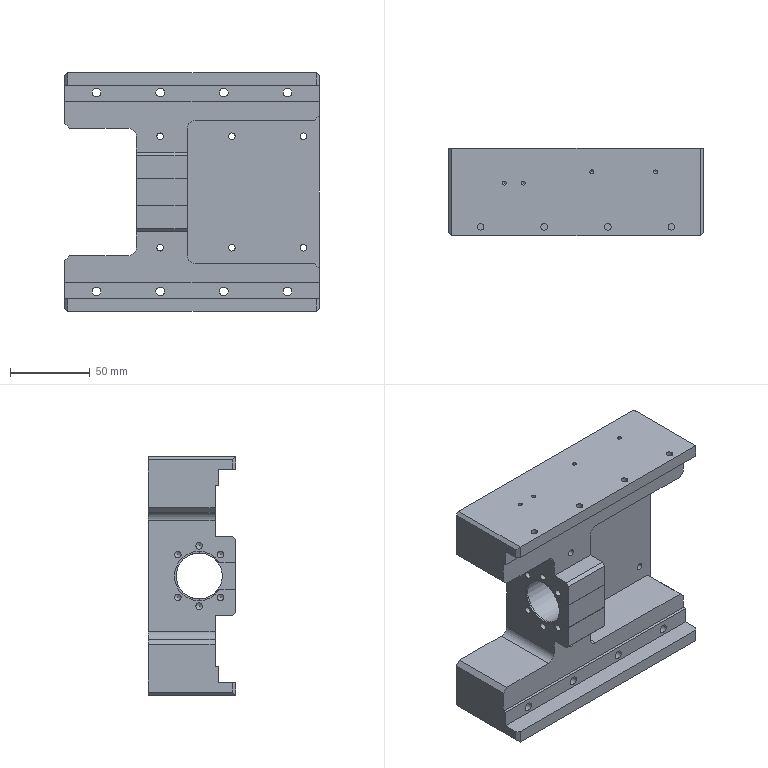CAM job | NX | 3+2 milling, drilling | part box 160 x 55 x 150 mm | stock box 165 x 60 x 155 mm
Tools:
number,name,description,diameter,corner_radius,flute_length,length,flutes
3,D3,平底铣刀-粗,3.0,0.0,20.0,75.0,2
6,D6,平底铣刀-粗,6.0,0.0,25.0,75.0,2
9,D10,平底铣刀-粗,10.0,0.0,35.0,75.0,2
17,D16,平底铣刀-粗,16.0,0.0,50.0,75.0,2
11,D3-J,平底铣刀-精,3.0,0.0,50.0,75.0,2
7,D6-J,平底铣刀-精,6.0,0.0,25.0,75.0,2
10,D10-J,平底铣刀-精,10.0,0.0,35.0,75.0,2
18,D16-J,平底铣刀-精,16.0,0.0,50.0,75.0,2
1,D80R0.8飞刀,圆鼻刀-粗,80.0,0.8,50.0,75.0,2
1,D80R0.8飞刀-J,圆鼻刀-精,80.0,0.8,50.0,75.0,2
2,D6倒角刀,倒角刀,6.0,0.0,3.0,25.0,2
19,D10倒角刀,倒角刀,10.0,0.0,5.0,75.0,2
22,M5X0.8,丝锥,4.2,0.0,35.0,50.0,2
18,ZT5.5,钻头,5.5,0.0,35.0,50.0,2
14,钻头4.2,Twist Drill 4.2 mm,4.2,0.0,41.0,41.738,2
17,ZT4.9,Drilling Tool,4.9,0.0,35.0,50.0,2
Operations:
program,operation,operation_type,tool,method,geometry_group,spindle_rpm,surface_speed,feed_per_tooth,feed_cut,feed_plunge,cut_length_mm,path_length_mm,cut_time_min,machine_time_min
C,等高往复层切开粗-中_COPY,ZLevelMilling,D16,分层开粗-切深K-步距G,W-C,5000.0,251.327,0.4,4000.0,100.0,5368.926,5564.926,1.342,1.362
C,打点-深0.8_2,Operation,D10倒角刀,NONE,W-C,5000.0,157.08,0.05,500.0,90.0,10.8,241.794,0.0216,0.0447
C,盲锥孔-M5螺纹底孔,Operation,钻头4.2,NONE,W-C,2500.0,32.987,0.03,150.0,90.0,87.971,396.136,0.5865,0.6173
C,铣倒角_4,PlanarMilling,D10倒角刀,METHOD,W-C,5000.0,157.08,0.05,500.0,100.0,86.111,959.558,0.1722,0.2596
C,底壁铣倒角_COPY_1,VolumeBased25DMillingOperation,D10倒角刀,爬面_倒角-切深0-步距G,W-C,5000.0,157.08,0.06,600.0,100.0,98.812,229.212,0.1647,0.1777
C,C0.3封闭铣廓倒角6X45L_COPY,PlanarMilling,D10倒角刀,爬面_倒角-切深0-步距G,W-C,7000.0,131.0,0.1071,1500.0,100.0,46.783,317.109,0.0312,0.0582
C,底壁铣精光侧面-中_COPY,VolumeBased25DMillingOperation,D16-J,侧刃精光-切深K-步距G,W-C,4000.0,201.062,0.125,1000.0,100.0,447.631,652.099,0.4476,0.4681
B,底壁铣飞面开粗_COPY,VolumeBased25DMillingOperation,D80R0.8飞刀,分层开粗-切深K-步距G,W-B,2800.0,703.696,0.5357,3000.0,100.0,7375.189,9819.447,2.458,2.703
B,底壁铣飞面精光_COPY,VolumeBased25DMillingOperation,D80R0.8飞刀-J,侧刃精光-切深K-步距G,W-B,4000.0,1005.28,0.125,1000.0,100.0,818.658,854.658,0.8187,0.8223
B,型腔铣开粗-中_COPY_1,CavityMilling,D10,分层开粗-切深K-步距G,W-B,8000.0,251.327,0.3125,5000.0,100.0,111828.209,119001.598,22.366,23.31
B,钻倒角_1,Operation,D6倒角刀,METHOD,W-B,8000.0,150.796,0.0625,1000.0,0.0,11.4,161.864,0.0114,0.0264
B,平面去毛刺6X45L_COPY,SurfaceContour,D6倒角刀,爬面_倒角-切深0-步距G,W-B,6500.0,122.519,0.1154,1500.0,100.0,1803.222,3831.172,1.202,1.405
B,底壁铣倒角_COPY,VolumeBased25DMillingOperation,D6倒角刀,爬面_倒角-切深0-步距G,W-B,6500.0,122.519,0.1154,1500.0,100.0,160.429,938.203,0.107,0.1847
B,底壁铣精光底面-中_COPY,VolumeBased25DMillingOperation,D10-J,精光步距切深关,W-B,7000.0,175.0,0.0536,1500.0,100.0,2464.717,2951.976,1.643,1.692
B,底壁铣精光底面-中_COPY_1,VolumeBased25DMillingOperation,D10-J,精光步距切深关,W-B,7000.0,175.0,0.0536,1500.0,100.0,1377.121,1487.121,0.9181,0.9291
B,底壁铣精光侧面-中-选底面_COPY,VolumeBased25DMillingOperation,D10-J,侧刃精光-切深K-步距G,W-B,8000.0,251.32,0.0625,1000.0,100.0,357.363,551.964,0.3574,0.3768
B,底壁铣精光侧面-中-选底面_COPY_1,VolumeBased25DMillingOperation,D10-J,侧刃精光-切深K-步距G,W-B,8000.0,251.32,0.0625,1000.0,100.0,458.726,737.423,0.4587,0.4866
B,底壁铣精光侧面-中-选底面_COPY_2,VolumeBased25DMillingOperation,D10-J,侧刃精光-切深K-步距G,W-B,8000.0,251.32,0.0625,1000.0,100.0,772.927,1043.502,0.7729,0.8
A,顶面,FaceMilling,D80R0.8飞刀,侧刃精光-切深K-步距G,W-A,4000.0,1005.31,0.125,1000.0,100.0,1112.0,1148.0,1.112,1.116
A,型腔铣开粗-中_COPY,CavityMilling,D10,分层开粗-切深K-步距G,W-A,6000.0,188.496,0.4167,5000.0,100.0,135221.252,139541.348,27.044,27.722
A,打点-深0.8,Operation,D6倒角刀,NONE,W-A,8000.0,150.796,0.0312,500.0,90.0,28.8,649.253,0.0576,0.1196
A,通孔-M5螺纹底孔,Operation,钻头4.2,NONE,W-A,3000.0,39.584,0.0583,350.0,90.0,185.571,666.193,0.5302,0.5783
A,通孔-精孔6.0预钻,Operation,ZT4.9,NONE,W-A,2500.0,38.484,0.05,250.0,90.0,16.889,164.784,0.0676,0.0823
A,沉头孔-钻孔0段,Operation,ZT5.5,NONE,W-A,1200.0,20.735,0.0625,150.0,90.0,389.219,1190.517,2.595,2.675
A,铣孔开粗D6_1,CylinderMilling,D6,NONE,W-A,8000.0,150.796,0.075,1200.0,100.0,5018.252,5899.252,4.182,4.27
A,铣孔精光D6_1,CylinderMilling,D6-J,精光步距切深关,W-A,8000.0,150.796,0.0312,500.0,100.0,691.319,1576.319,1.383,1.471
A,铣孔开粗D4_1,CylinderMilling,D3,NONE,W-A,8000.0,75.398,0.0312,500.0,100.0,273.984,454.984,0.548,0.5661
A,外形粗_2,VolumeBased25DMillingOperation,D10,METHOD,W-A,8000.0,251.327,0.3125,5000.0,80.0,51793.571,51887.071,10.359,10.368
A,仅选体,SurfaceContour,D6倒角刀,METHOD,W-A,8000.0,150.796,0.1875,3000.0,100.0,714.802,750.603,0.2383,0.2418
A,铣倒角_1,PlanarMilling,D6倒角刀,METHOD,W-A,8000.0,150.796,0.0312,500.0,100.0,108.122,604.136,0.2162,0.2658
A,铣倒角_2,PlanarMilling,D6倒角刀,METHOD,W-A,8000.0,150.796,0.0312,500.0,100.0,36.963,207.394,0.0739,0.091
A,铣倒角_3,PlanarMilling,D6倒角刀,NONE,W-A,8000.0,150.796,0.05,800.0,100.0,322.008,971.75,0.4025,0.4675
A,通孔-攻牙M5,Operation,M5X0.8,METHOD,W-A,500.0,6.597,0.0008,0.8,90.0,70.0,343.029,87.5,87.527
A,铣孔精光D4-J_1,CylinderMilling,D3-J,精光步距切深关,W-A,8000.0,75.398,0.0125,200.0,100.0,102.347,283.347,0.5117,0.5298
A,外形半精_2,VolumeBased25DMillingOperation,D10-J,METHOD,W-A,5000.0,157.08,0.1,1000.0,100.0,4403.286,5036.259,4.403,4.467